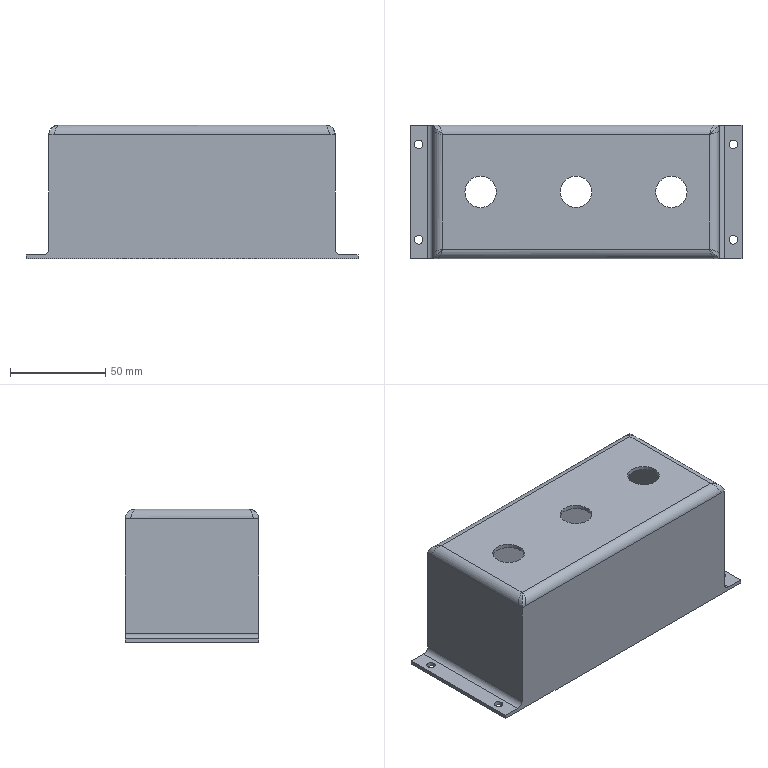Part | STEP file | Clip connector box | 1 solid | 57 faces | box 174 x 70 x 70 mm | volume 79761 mm3 | cylinder 26 | spline 16 | plane 15 | commonest cylinder face diameters 4.5 x8 6 x6 10 x6 16.5 x6